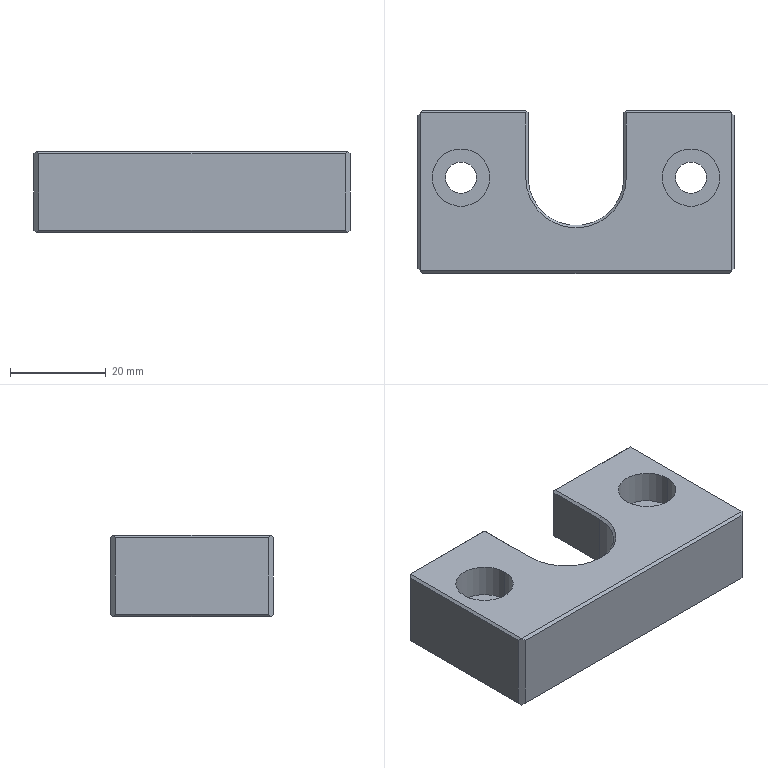Part | STEP file | 03-31SC Floating JointFixed座 | 1 solid | 51 faces | box 66 x 34 x 17 mm | volume 26495 mm3 | plane 38 | cylinder 10 | cone 3 | commonest cylinder face diameters 6.5 x4 12 x4 20 x1 31 x1
STEP:
#1=CARTESIAN_POINT('',(-30.,3.,10.));
#2=VERTEX_POINT('',#1);
#3=CARTESIAN_POINT('',(-18.,3.,10.));
#4=VERTEX_POINT('',#3);
#5=CARTESIAN_POINT('',(-24.,3.,10.));
#6=DIRECTION('',(0.,0.,1.));
#7=DIRECTION('',(1.,0.,0.));
#8=AXIS2_PLACEMENT_3D('',#5,#6,#7);
#9=CIRCLE('',#8,6.);
#10=EDGE_CURVE('',#2,#4,#9,.T.);
#11=ORIENTED_EDGE('',*,*,#10,.F.);
#12=CARTESIAN_POINT('',(-30.,3.,17.));
#13=VERTEX_POINT('',#12);
#14=CARTESIAN_POINT('',(-30.,3.,17.));
#15=DIRECTION('',(0.,0.,1.));
#16=VECTOR('',#15,1000.);
#17=LINE('',#14,#16);
#18=EDGE_CURVE('',#2,#13,#17,.T.);
#19=ORIENTED_EDGE('',*,*,#18,.T.);
#20=CARTESIAN_POINT('',(-18.,3.,17.));
#21=VERTEX_POINT('',#20);
#22=CARTESIAN_POINT('',(-24.,3.,17.));
#23=DIRECTION('',(0.,0.,1.));
#24=DIRECTION('',(1.,0.,0.));
#25=AXIS2_PLACEMENT_3D('',#22,#23,#24);
#26=CIRCLE('',#25,6.);
#27=EDGE_CURVE('',#13,#21,#26,.T.);
#28=ORIENTED_EDGE('',*,*,#27,.T.);
#29=CARTESIAN_POINT('',(-18.,3.,17.));
#30=DIRECTION('',(0.,0.,1.));
#31=VECTOR('',#30,1000.);
#32=LINE('',#29,#31);
#33=EDGE_CURVE('',#4,#21,#32,.T.);
#34=ORIENTED_EDGE('',*,*,#33,.F.);
#35=EDGE_LOOP('',(#11,#19,#28,#34));
#36=FACE_OUTER_BOUND('',#35,.T.);
#37=CARTESIAN_POINT('',(-24.,3.,17.));
#38=DIRECTION('',(0.,0.,1.));
#39=DIRECTION('',(1.,0.,0.));
#40=AXIS2_PLACEMENT_3D('',#37,#38,#39);
#41=CYLINDRICAL_SURFACE('',#40,6.);
#42=ADVANCED_FACE('',(#36),#41,.F.);
#43=CARTESIAN_POINT('',(-27.25,3.,0.));
#44=VERTEX_POINT('',#43);
#45=CARTESIAN_POINT('',(-20.75,3.,0.));
#46=VERTEX_POINT('',#45);
#47=CARTESIAN_POINT('',(-24.,3.,0.));
#48=DIRECTION('',(0.,0.,1.));
#49=DIRECTION('',(1.,0.,0.));
#50=AXIS2_PLACEMENT_3D('',#47,#48,#49);
#51=CIRCLE('',#50,3.25);
#52=EDGE_CURVE('',#44,#46,#51,.T.);
#53=ORIENTED_EDGE('',*,*,#52,.F.);
#54=CARTESIAN_POINT('',(-27.25,3.,10.));
#55=VERTEX_POINT('',#54);
#56=CARTESIAN_POINT('',(-27.25,3.,17.));
#57=DIRECTION('',(0.,0.,1.));
#58=VECTOR('',#57,1000.);
#59=LINE('',#56,#58);
#60=EDGE_CURVE('',#44,#55,#59,.T.);
#61=ORIENTED_EDGE('',*,*,#60,.T.);
#62=CARTESIAN_POINT('',(-20.75,3.,10.));
#63=VERTEX_POINT('',#62);
#64=CARTESIAN_POINT('',(-24.,3.,10.));
#65=DIRECTION('',(0.,0.,1.));
#66=DIRECTION('',(1.,0.,0.));
#67=AXIS2_PLACEMENT_3D('',#64,#65,#66);
#68=CIRCLE('',#67,3.25);
#69=EDGE_CURVE('',#55,#63,#68,.T.);
#70=ORIENTED_EDGE('',*,*,#69,.T.);
#71=CARTESIAN_POINT('',(-20.75,3.,17.));
#72=DIRECTION('',(0.,0.,1.));
#73=VECTOR('',#72,1000.);
#74=LINE('',#71,#73);
#75=EDGE_CURVE('',#46,#63,#74,.T.);
#76=ORIENTED_EDGE('',*,*,#75,.F.);
#77=EDGE_LOOP('',(#53,#61,#70,#76));
#78=FACE_OUTER_BOUND('',#77,.T.);
#79=CARTESIAN_POINT('',(-24.,3.,17.));
#80=DIRECTION('',(0.,0.,1.));
#81=DIRECTION('',(1.,0.,0.));
#82=AXIS2_PLACEMENT_3D('',#79,#80,#81);
#83=CYLINDRICAL_SURFACE('',#82,3.25);
#84=ADVANCED_FACE('',(#78),#83,.F.);
#85=CARTESIAN_POINT('',(18.,3.,10.));
#86=VERTEX_POINT('',#85);
#87=CARTESIAN_POINT('',(30.,3.,10.));
#88=VERTEX_POINT('',#87);
#89=CARTESIAN_POINT('',(24.,3.,10.));
#90=DIRECTION('',(0.,0.,1.));
#91=DIRECTION('',(1.,0.,0.));
#92=AXIS2_PLACEMENT_3D('',#89,#90,#91);
#93=CIRCLE('',#92,6.);
#94=EDGE_CURVE('',#86,#88,#93,.T.);
#95=ORIENTED_EDGE('',*,*,#94,.F.);
#96=CARTESIAN_POINT('',(18.,3.,17.));
#97=VERTEX_POINT('',#96);
#98=CARTESIAN_POINT('',(18.,3.,17.));
#99=DIRECTION('',(0.,0.,1.));
#100=VECTOR('',#99,1000.);
#101=LINE('',#98,#100);
#102=EDGE_CURVE('',#86,#97,#101,.T.);
#103=ORIENTED_EDGE('',*,*,#102,.T.);
#104=CARTESIAN_POINT('',(30.,3.,17.));
#105=VERTEX_POINT('',#104);
#106=CARTESIAN_POINT('',(24.,3.,17.));
#107=DIRECTION('',(0.,0.,1.));
#108=DIRECTION('',(1.,0.,0.));
#109=AXIS2_PLACEMENT_3D('',#106,#107,#108);
#110=CIRCLE('',#109,6.);
#111=EDGE_CURVE('',#97,#105,#110,.T.);
#112=ORIENTED_EDGE('',*,*,#111,.T.);
#113=CARTESIAN_POINT('',(30.,3.,17.));
#114=DIRECTION('',(0.,0.,1.));
#115=VECTOR('',#114,1000.);
#116=LINE('',#113,#115);
#117=EDGE_CURVE('',#88,#105,#116,.T.);
#118=ORIENTED_EDGE('',*,*,#117,.F.);
#119=EDGE_LOOP('',(#95,#103,#112,#118));
#120=FACE_OUTER_BOUND('',#119,.T.);
#121=CARTESIAN_POINT('',(24.,3.,17.));
#122=DIRECTION('',(0.,0.,1.));
#123=DIRECTION('',(1.,0.,0.));
#124=AXIS2_PLACEMENT_3D('',#121,#122,#123);
#125=CYLINDRICAL_SURFACE('',#124,6.);
#126=ADVANCED_FACE('',(#120),#125,.F.);
#127=CARTESIAN_POINT('',(20.75,3.,0.));
#128=VERTEX_POINT('',#127);
#129=CARTESIAN_POINT('',(27.25,3.,0.));
#130=VERTEX_POINT('',#129);
#131=CARTESIAN_POINT('',(24.,3.,0.));
#132=DIRECTION('',(0.,0.,1.));
#133=DIRECTION('',(1.,0.,0.));
#134=AXIS2_PLACEMENT_3D('',#131,#132,#133);
#135=CIRCLE('',#134,3.25);
#136=EDGE_CURVE('',#128,#130,#135,.T.);
#137=ORIENTED_EDGE('',*,*,#136,.F.);
#138=CARTESIAN_POINT('',(20.75,3.,10.));
#139=VERTEX_POINT('',#138);
#140=CARTESIAN_POINT('',(20.75,3.,17.));
#141=DIRECTION('',(0.,0.,1.));
#142=VECTOR('',#141,1000.);
#143=LINE('',#140,#142);
#144=EDGE_CURVE('',#128,#139,#143,.T.);
#145=ORIENTED_EDGE('',*,*,#144,.T.);
#146=CARTESIAN_POINT('',(27.25,3.,10.));
#147=VERTEX_POINT('',#146);
#148=CARTESIAN_POINT('',(24.,3.,10.));
#149=DIRECTION('',(0.,0.,1.));
#150=DIRECTION('',(1.,0.,0.));
#151=AXIS2_PLACEMENT_3D('',#148,#149,#150);
#152=CIRCLE('',#151,3.25);
#153=EDGE_CURVE('',#139,#147,#152,.T.);
#154=ORIENTED_EDGE('',*,*,#153,.T.);
#155=CARTESIAN_POINT('',(27.25,3.,17.));
#156=DIRECTION('',(0.,0.,1.));
#157=VECTOR('',#156,1000.);
#158=LINE('',#155,#157);
#159=EDGE_CURVE('',#130,#147,#158,.T.);
#160=ORIENTED_EDGE('',*,*,#159,.F.);
#161=EDGE_LOOP('',(#137,#145,#154,#160));
#162=FACE_OUTER_BOUND('',#161,.T.);
#163=CARTESIAN_POINT('',(24.,3.,17.));
#164=DIRECTION('',(0.,0.,1.));
#165=DIRECTION('',(1.,0.,0.));
#166=AXIS2_PLACEMENT_3D('',#163,#164,#165);
#167=CYLINDRICAL_SURFACE('',#166,3.25);
#168=ADVANCED_FACE('',(#162),#167,.F.);
#169=CARTESIAN_POINT('',(10.5,17.,5.));
#170=VERTEX_POINT('',#169);
#171=CARTESIAN_POINT('',(10.5,17.,16.5));
#172=VERTEX_POINT('',#171);
#173=CARTESIAN_POINT('',(10.5,17.,0.));
#174=DIRECTION('',(0.,0.,1.));
#175=VECTOR('',#174,1000.);
#176=LINE('',#173,#175);
#177=EDGE_CURVE('',#170,#172,#176,.T.);
#178=ORIENTED_EDGE('',*,*,#177,.T.);
#179=CARTESIAN_POINT('',(32.,17.,16.5));
#180=VERTEX_POINT('',#179);
#181=CARTESIAN_POINT('',(32.,17.,16.5));
#182=DIRECTION('',(1.,0.,0.));
#183=VECTOR('',#182,1000.);
#184=LINE('',#181,#183);
#185=EDGE_CURVE('',#172,#180,#184,.T.);
#186=ORIENTED_EDGE('',*,*,#185,.T.);
#187=CARTESIAN_POINT('',(32.,17.,0.5));
#188=VERTEX_POINT('',#187);
#189=CARTESIAN_POINT('',(32.,17.,17.));
#190=DIRECTION('',(0.,0.,-1.));
#191=VECTOR('',#190,1000.);
#192=LINE('',#189,#191);
#193=EDGE_CURVE('',#180,#188,#192,.T.);
#194=ORIENTED_EDGE('',*,*,#193,.T.);
#195=CARTESIAN_POINT('',(16.,17.,0.5));
#196=VERTEX_POINT('',#195);
#197=CARTESIAN_POINT('',(-32.,17.,0.5));
#198=DIRECTION('',(-1.,0.,0.));
#199=VECTOR('',#198,1000.);
#200=LINE('',#197,#199);
#201=EDGE_CURVE('',#188,#196,#200,.T.);
#202=ORIENTED_EDGE('',*,*,#201,.T.);
#203=CARTESIAN_POINT('',(16.,17.,5.));
#204=VERTEX_POINT('',#203);
#205=CARTESIAN_POINT('',(16.,17.,5.));
#206=DIRECTION('',(0.,0.,1.));
#207=VECTOR('',#206,1000.);
#208=LINE('',#205,#207);
#209=EDGE_CURVE('',#196,#204,#208,.T.);
#210=ORIENTED_EDGE('',*,*,#209,.T.);
#211=CARTESIAN_POINT('',(-15.5,17.,5.));
#212=DIRECTION('',(1.,0.,0.));
#213=VECTOR('',#212,1000.);
#214=LINE('',#211,#213);
#215=EDGE_CURVE('',#170,#204,#214,.T.);
#216=ORIENTED_EDGE('',*,*,#215,.F.);
#217=EDGE_LOOP('',(#178,#186,#194,#202,#210,#216));
#218=FACE_OUTER_BOUND('',#217,.T.);
#219=CARTESIAN_POINT('',(-32.,17.,17.));
#220=DIRECTION('',(0.,1.,0.));
#221=DIRECTION('',(-1.,0.,0.));
#222=AXIS2_PLACEMENT_3D('',#219,#220,#221);
#223=PLANE('',#222);
#224=ADVANCED_FACE('',(#218),#223,.T.);
#225=CARTESIAN_POINT('',(-32.,17.,16.5));
#226=VERTEX_POINT('',#225);
#227=CARTESIAN_POINT('',(-32.,17.,0.5));
#228=VERTEX_POINT('',#227);
#229=CARTESIAN_POINT('',(-32.,17.,17.));
#230=DIRECTION('',(0.,0.,-1.));
#231=VECTOR('',#230,1000.);
#232=LINE('',#229,#231);
#233=EDGE_CURVE('',#226,#228,#232,.T.);
#234=ORIENTED_EDGE('',*,*,#233,.T.);
#235=CARTESIAN_POINT('',(-32.5,16.5,0.));
#236=VERTEX_POINT('',#235);
#237=CARTESIAN_POINT('',(-27.167,21.833,5.333));
#238=DIRECTION('',(-0.5774,-0.5774,-0.5774));
#239=VECTOR('',#238,1000.);
#240=LINE('',#237,#239);
#241=EDGE_CURVE('',#228,#236,#240,.T.);
#242=ORIENTED_EDGE('',*,*,#241,.T.);
#243=CARTESIAN_POINT('',(-33.,16.,0.5));
#244=VERTEX_POINT('',#243);
#245=CARTESIAN_POINT('',(-38.5,10.5,6.));
#246=DIRECTION('',(-0.5774,-0.5774,0.5774));
#247=VECTOR('',#246,1000.);
#248=LINE('',#245,#247);
#249=EDGE_CURVE('',#236,#244,#248,.T.);
#250=ORIENTED_EDGE('',*,*,#249,.T.);
#251=CARTESIAN_POINT('',(-33.,16.,16.5));
#252=VERTEX_POINT('',#251);
#253=CARTESIAN_POINT('',(-33.,16.,17.));
#254=DIRECTION('',(0.,0.,-1.));
#255=VECTOR('',#254,1000.);
#256=LINE('',#253,#255);
#257=EDGE_CURVE('',#252,#244,#256,.T.);
#258=ORIENTED_EDGE('',*,*,#257,.F.);
#259=CARTESIAN_POINT('',(-32.5,16.5,17.));
#260=VERTEX_POINT('',#259);
#261=CARTESIAN_POINT('',(-32.833,16.167,16.667));
#262=DIRECTION('',(0.5774,0.5774,0.5774));
#263=VECTOR('',#262,1000.);
#264=LINE('',#261,#263);
#265=EDGE_CURVE('',#252,#260,#264,.T.);
#266=ORIENTED_EDGE('',*,*,#265,.T.);
#267=CARTESIAN_POINT('',(-32.833,16.167,17.333));
#268=DIRECTION('',(0.5774,0.5774,-0.5774));
#269=VECTOR('',#268,1000.);
#270=LINE('',#267,#269);
#271=EDGE_CURVE('',#260,#226,#270,.T.);
#272=ORIENTED_EDGE('',*,*,#271,.T.);
#273=EDGE_LOOP('',(#234,#242,#250,#258,#266,#272));
#274=FACE_OUTER_BOUND('',#273,.T.);
#275=CARTESIAN_POINT('',(-33.,16.,17.));
#276=DIRECTION('',(-0.7071,0.7071,0.));
#277=DIRECTION('',(-0.7071,-0.7071,0.));
#278=AXIS2_PLACEMENT_3D('',#275,#276,#277);
#279=PLANE('',#278);
#280=ADVANCED_FACE('',(#274),#279,.T.);
#281=ORIENTED_EDGE('',*,*,#257,.T.);
#282=CARTESIAN_POINT('',(-33.,-16.,0.5));
#283=VERTEX_POINT('',#282);
#284=CARTESIAN_POINT('',(-33.,-16.,0.5));
#285=DIRECTION('',(0.,-1.,0.));
#286=VECTOR('',#285,1000.);
#287=LINE('',#284,#286);
#288=EDGE_CURVE('',#244,#283,#287,.T.);
#289=ORIENTED_EDGE('',*,*,#288,.T.);
#290=CARTESIAN_POINT('',(-33.,-16.,16.5));
#291=VERTEX_POINT('',#290);
#292=CARTESIAN_POINT('',(-33.,-16.,17.));
#293=DIRECTION('',(0.,0.,-1.));
#294=VECTOR('',#293,1000.);
#295=LINE('',#292,#294);
#296=EDGE_CURVE('',#291,#283,#295,.T.);
#297=ORIENTED_EDGE('',*,*,#296,.F.);
#298=CARTESIAN_POINT('',(-33.,16.,16.5));
#299=DIRECTION('',(0.,1.,0.));
#300=VECTOR('',#299,1000.);
#301=LINE('',#298,#300);
#302=EDGE_CURVE('',#291,#252,#301,.T.);
#303=ORIENTED_EDGE('',*,*,#302,.T.);
#304=EDGE_LOOP('',(#281,#289,#297,#303));
#305=FACE_OUTER_BOUND('',#304,.T.);
#306=CARTESIAN_POINT('',(-33.,-16.,17.));
#307=DIRECTION('',(-1.,0.,0.));
#308=DIRECTION('',(0.,0.,1.));
#309=AXIS2_PLACEMENT_3D('',#306,#307,#308);
#310=PLANE('',#309);
#311=ADVANCED_FACE('',(#305),#310,.T.);
#312=CARTESIAN_POINT('',(-32.,-17.,16.5));
#313=VERTEX_POINT('',#312);
#314=CARTESIAN_POINT('',(-32.,-17.,0.5));
#315=VERTEX_POINT('',#314);
#316=CARTESIAN_POINT('',(-32.,-17.,17.));
#317=DIRECTION('',(0.,0.,-1.));
#318=VECTOR('',#317,1000.);
#319=LINE('',#316,#318);
#320=EDGE_CURVE('',#313,#315,#319,.T.);
#321=ORIENTED_EDGE('',*,*,#320,.F.);
#322=CARTESIAN_POINT('',(-32.5,-16.5,17.));
#323=VERTEX_POINT('',#322);
#324=CARTESIAN_POINT('',(-32.167,-16.833,16.667));
#325=DIRECTION('',(-0.5774,0.5774,0.5774));
#326=VECTOR('',#325,1000.);
#327=LINE('',#324,#326);
#328=EDGE_CURVE('',#313,#323,#327,.T.);
#329=ORIENTED_EDGE('',*,*,#328,.T.);
#330=CARTESIAN_POINT('',(-32.167,-16.833,17.333));
#331=DIRECTION('',(-0.5774,0.5774,-0.5774));
#332=VECTOR('',#331,1000.);
#333=LINE('',#330,#332);
#334=EDGE_CURVE('',#323,#291,#333,.T.);
#335=ORIENTED_EDGE('',*,*,#334,.T.);
#336=ORIENTED_EDGE('',*,*,#296,.T.);
#337=CARTESIAN_POINT('',(-32.5,-16.5,0.));
#338=VERTEX_POINT('',#337);
#339=CARTESIAN_POINT('',(-37.833,-11.167,5.333));
#340=DIRECTION('',(0.5774,-0.5774,-0.5774));
#341=VECTOR('',#340,1000.);
#342=LINE('',#339,#341);
#343=EDGE_CURVE('',#283,#338,#342,.T.);
#344=ORIENTED_EDGE('',*,*,#343,.T.);
#345=CARTESIAN_POINT('',(-26.5,-22.5,6.));
#346=DIRECTION('',(0.5774,-0.5774,0.5774));
#347=VECTOR('',#346,1000.);
#348=LINE('',#345,#347);
#349=EDGE_CURVE('',#338,#315,#348,.T.);
#350=ORIENTED_EDGE('',*,*,#349,.T.);
#351=EDGE_LOOP('',(#321,#329,#335,#336,#344,#350));
#352=FACE_OUTER_BOUND('',#351,.T.);
#353=CARTESIAN_POINT('',(-32.,-17.,17.));
#354=DIRECTION('',(-0.7071,-0.7071,0.));
#355=DIRECTION('',(0.7071,-0.7071,0.));
#356=AXIS2_PLACEMENT_3D('',#353,#354,#355);
#357=PLANE('',#356);
#358=ADVANCED_FACE('',(#352),#357,.T.);
#359=CARTESIAN_POINT('',(32.,-17.,16.5));
#360=VERTEX_POINT('',#359);
#361=CARTESIAN_POINT('',(32.,-17.,0.5));
#362=VERTEX_POINT('',#361);
#363=CARTESIAN_POINT('',(32.,-17.,17.));
#364=DIRECTION('',(0.,0.,-1.));
#365=VECTOR('',#364,1000.);
#366=LINE('',#363,#365);
#367=EDGE_CURVE('',#360,#362,#366,.T.);
#368=ORIENTED_EDGE('',*,*,#367,.F.);
#369=CARTESIAN_POINT('',(-32.,-17.,16.5));
#370=DIRECTION('',(-1.,0.,0.));
#371=VECTOR('',#370,1000.);
#372=LINE('',#369,#371);
#373=EDGE_CURVE('',#360,#313,#372,.T.);
#374=ORIENTED_EDGE('',*,*,#373,.T.);
#375=ORIENTED_EDGE('',*,*,#320,.T.);
#376=CARTESIAN_POINT('',(32.,-17.,0.5));
#377=DIRECTION('',(1.,0.,0.));
#378=VECTOR('',#377,1000.);
#379=LINE('',#376,#378);
#380=EDGE_CURVE('',#315,#362,#379,.T.);
#381=ORIENTED_EDGE('',*,*,#380,.T.);
#382=EDGE_LOOP('',(#368,#374,#375,#381));
#383=FACE_OUTER_BOUND('',#382,.T.);
#384=CARTESIAN_POINT('',(32.,-17.,17.));
#385=DIRECTION('',(0.,-1.,0.));
#386=DIRECTION('',(1.,0.,0.));
#387=AXIS2_PLACEMENT_3D('',#384,#385,#386);
#388=PLANE('',#387);
#389=ADVANCED_FACE('',(#383),#388,.T.);
#390=CARTESIAN_POINT('',(33.,-16.,16.5));
#391=VERTEX_POINT('',#390);
#392=CARTESIAN_POINT('',(32.5,-16.5,17.));
#393=VERTEX_POINT('',#392);
#394=CARTESIAN_POINT('',(32.833,-16.167,16.667));
#395=DIRECTION('',(-0.5774,-0.5774,0.5774));
#396=VECTOR('',#395,1000.);
#397=LINE('',#394,#396);
#398=EDGE_CURVE('',#391,#393,#397,.T.);
#399=ORIENTED_EDGE('',*,*,#398,.T.);
#400=CARTESIAN_POINT('',(32.833,-16.167,17.333));
#401=DIRECTION('',(-0.5774,-0.5774,-0.5774));
#402=VECTOR('',#401,1000.);
#403=LINE('',#400,#402);
#404=EDGE_CURVE('',#393,#360,#403,.T.);
#405=ORIENTED_EDGE('',*,*,#404,.T.);
#406=ORIENTED_EDGE('',*,*,#367,.T.);
#407=CARTESIAN_POINT('',(32.5,-16.5,0.));
#408=VERTEX_POINT('',#407);
#409=CARTESIAN_POINT('',(27.167,-21.833,5.333));
#410=DIRECTION('',(0.5774,0.5774,-0.5774));
#411=VECTOR('',#410,1000.);
#412=LINE('',#409,#411);
#413=EDGE_CURVE('',#362,#408,#412,.T.);
#414=ORIENTED_EDGE('',*,*,#413,.T.);
#415=CARTESIAN_POINT('',(33.,-16.,0.5));
#416=VERTEX_POINT('',#415);
#417=CARTESIAN_POINT('',(38.5,-10.5,6.));
#418=DIRECTION('',(0.5774,0.5774,0.5774));
#419=VECTOR('',#418,1000.);
#420=LINE('',#417,#419);
#421=EDGE_CURVE('',#408,#416,#420,.T.);
#422=ORIENTED_EDGE('',*,*,#421,.T.);
#423=CARTESIAN_POINT('',(33.,-16.,17.));
#424=DIRECTION('',(0.,0.,-1.));
#425=VECTOR('',#424,1000.);
#426=LINE('',#423,#425);
#427=EDGE_CURVE('',#391,#416,#426,.T.);
#428=ORIENTED_EDGE('',*,*,#427,.F.);
#429=EDGE_LOOP('',(#399,#405,#406,#414,#422,#428));
#430=FACE_OUTER_BOUND('',#429,.T.);
#431=CARTESIAN_POINT('',(33.,-16.,17.));
#432=DIRECTION('',(0.7071,-0.7071,0.));
#433=DIRECTION('',(0.7071,0.7071,0.));
#434=AXIS2_PLACEMENT_3D('',#431,#432,#433);
#435=PLANE('',#434);
#436=ADVANCED_FACE('',(#430),#435,.T.);
#437=CARTESIAN_POINT('',(33.,16.,16.5));
#438=VERTEX_POINT('',#437);
#439=CARTESIAN_POINT('',(33.,16.,0.5));
#440=VERTEX_POINT('',#439);
#441=CARTESIAN_POINT('',(33.,16.,17.));
#442=DIRECTION('',(0.,0.,-1.));
#443=VECTOR('',#442,1000.);
#444=LINE('',#441,#443);
#445=EDGE_CURVE('',#438,#440,#444,.T.);
#446=ORIENTED_EDGE('',*,*,#445,.F.);
#447=CARTESIAN_POINT('',(33.,-16.,16.5));
#448=DIRECTION('',(0.,-1.,0.));
#449=VECTOR('',#448,1000.);
#450=LINE('',#447,#449);
#451=EDGE_CURVE('',#438,#391,#450,.T.);
#452=ORIENTED_EDGE('',*,*,#451,.T.);
#453=ORIENTED_EDGE('',*,*,#427,.T.);
#454=CARTESIAN_POINT('',(33.,16.,0.5));
#455=DIRECTION('',(0.,1.,0.));
#456=VECTOR('',#455,1000.);
#457=LINE('',#454,#456);
#458=EDGE_CURVE('',#416,#440,#457,.T.);
#459=ORIENTED_EDGE('',*,*,#458,.T.);
#460=EDGE_LOOP('',(#446,#452,#453,#459));
#461=FACE_OUTER_BOUND('',#460,.T.);
#462=CARTESIAN_POINT('',(33.,16.,17.));
#463=DIRECTION('',(1.,0.,0.));
#464=DIRECTION('',(0.,0.,-1.));
#465=AXIS2_PLACEMENT_3D('',#462,#463,#464);
#466=PLANE('',#465);
#467=ADVANCED_FACE('',(#461),#466,.T.);
#468=ORIENTED_EDGE('',*,*,#193,.F.);
#469=CARTESIAN_POINT('',(32.5,16.5,17.));
#470=VERTEX_POINT('',#469);
#471=CARTESIAN_POINT('',(32.167,16.833,16.667));
#472=DIRECTION('',(0.5774,-0.5774,0.5774));
#473=VECTOR('',#472,1000.);
#474=LINE('',#471,#473);
#475=EDGE_CURVE('',#180,#470,#474,.T.);
#476=ORIENTED_EDGE('',*,*,#475,.T.);
#477=CARTESIAN_POINT('',(32.167,16.833,17.333));
#478=DIRECTION('',(0.5774,-0.5774,-0.5774));
#479=VECTOR('',#478,1000.);
#480=LINE('',#477,#479);
#481=EDGE_CURVE('',#470,#438,#480,.T.);
#482=ORIENTED_EDGE('',*,*,#481,.T.);
#483=ORIENTED_EDGE('',*,*,#445,.T.);
#484=CARTESIAN_POINT('',(32.5,16.5,0.));
#485=VERTEX_POINT('',#484);
#486=CARTESIAN_POINT('',(37.833,11.167,5.333));
#487=DIRECTION('',(-0.5774,0.5774,-0.5774));
#488=VECTOR('',#487,1000.);
#489=LINE('',#486,#488);
#490=EDGE_CURVE('',#440,#485,#489,.T.);
#491=ORIENTED_EDGE('',*,*,#490,.T.);
#492=CARTESIAN_POINT('',(26.5,22.5,6.));
#493=DIRECTION('',(-0.5774,0.5774,0.5774));
#494=VECTOR('',#493,1000.);
#495=LINE('',#492,#494);
#496=EDGE_CURVE('',#485,#188,#495,.T.);
#497=ORIENTED_EDGE('',*,*,#496,.T.);
#498=EDGE_LOOP('',(#468,#476,#482,#483,#491,#497));
#499=FACE_OUTER_BOUND('',#498,.T.);
#500=CARTESIAN_POINT('',(32.,17.,17.));
#501=DIRECTION('',(0.7071,0.7071,0.));
#502=DIRECTION('',(-0.7071,0.7071,0.));
#503=AXIS2_PLACEMENT_3D('',#500,#501,#502);
#504=PLANE('',#503);
#505=ADVANCED_FACE('',(#499),#504,.T.);
#506=ORIENTED_EDGE('',*,*,#233,.F.);
#507=CARTESIAN_POINT('',(-10.5,17.,16.5));
#508=VERTEX_POINT('',#507);
#509=CARTESIAN_POINT('',(-10.5,17.,16.5));
#510=DIRECTION('',(1.,0.,0.));
#511=VECTOR('',#510,1000.);
#512=LINE('',#509,#511);
#513=EDGE_CURVE('',#226,#508,#512,.T.);
#514=ORIENTED_EDGE('',*,*,#513,.T.);
#515=CARTESIAN_POINT('',(-10.5,17.,5.));
#516=VERTEX_POINT('',#515);
#517=CARTESIAN_POINT('',(-10.5,17.,0.));
#518=DIRECTION('',(0.,0.,1.));
#519=VECTOR('',#518,1000.);
#520=LINE('',#517,#519);
#521=EDGE_CURVE('',#516,#508,#520,.T.);
#522=ORIENTED_EDGE('',*,*,#521,.F.);
#523=CARTESIAN_POINT('',(-16.,17.,5.));
#524=VERTEX_POINT('',#523);
#525=CARTESIAN_POINT('',(-15.5,17.,5.));
#526=DIRECTION('',(1.,0.,0.));
#527=VECTOR('',#526,1000.);
#528=LINE('',#525,#527);
#529=EDGE_CURVE('',#524,#516,#528,.T.);
#530=ORIENTED_EDGE('',*,*,#529,.F.);
#531=CARTESIAN_POINT('',(-16.,17.,0.5));
#532=VERTEX_POINT('',#531);
#533=CARTESIAN_POINT('',(-16.,17.,0.));
#534=DIRECTION('',(0.,0.,-1.));
#535=VECTOR('',#534,1000.);
#536=LINE('',#533,#535);
#537=EDGE_CURVE('',#524,#532,#536,.T.);
#538=ORIENTED_EDGE('',*,*,#537,.T.);
#539=CARTESIAN_POINT('',(-32.,17.,0.5));
#540=DIRECTION('',(-1.,0.,0.));
#541=VECTOR('',#540,1000.);
#542=LINE('',#539,#541);
#543=EDGE_CURVE('',#532,#228,#542,.T.);
#544=ORIENTED_EDGE('',*,*,#543,.T.);
#545=EDGE_LOOP('',(#506,#514,#522,#530,#538,#544));
#546=FACE_OUTER_BOUND('',#545,.T.);
#547=CARTESIAN_POINT('',(-32.,17.,17.));
#548=DIRECTION('',(0.,1.,0.));
#549=DIRECTION('',(-1.,0.,0.));
#550=AXIS2_PLACEMENT_3D('',#547,#548,#549);
#551=PLANE('',#550);
#552=ADVANCED_FACE('',(#546),#551,.T.);
#553=CARTESIAN_POINT('',(10.5,16.5,17.));
#554=VERTEX_POINT('',#553);
#555=CARTESIAN_POINT('',(10.5,16.5,17.));
#556=DIRECTION('',(-1.,0.,0.));
#557=VECTOR('',#556,1000.);
#558=LINE('',#555,#557);
#559=EDGE_CURVE('',#470,#554,#558,.T.);
#560=ORIENTED_EDGE('',*,*,#559,.T.);
#561=CARTESIAN_POINT('',(10.5,3.,17.));
#562=VERTEX_POINT('',#561);
#563=CARTESIAN_POINT('',(10.5,49.,17.));
#564=DIRECTION('',(0.,-1.,0.));
#565=VECTOR('',#564,1000.);
#566=LINE('',#563,#565);
#567=EDGE_CURVE('',#554,#562,#566,.T.);
#568=ORIENTED_EDGE('',*,*,#567,.T.);
#569=CARTESIAN_POINT('',(-10.5,3.,17.));
#570=VERTEX_POINT('',#569);
#571=CARTESIAN_POINT('',(0.,3.,17.));
#572=DIRECTION('',(0.,0.,-1.));
#573=DIRECTION('',(-1.,0.,0.));
#574=AXIS2_PLACEMENT_3D('',#571,#572,#573);
#575=CIRCLE('',#574,10.5);
#576=EDGE_CURVE('',#562,#570,#575,.T.);
#577=ORIENTED_EDGE('',*,*,#576,.T.);
#578=CARTESIAN_POINT('',(-10.5,16.5,17.));
#579=VERTEX_POINT('',#578);
#580=CARTESIAN_POINT('',(-10.5,49.,17.));
#581=DIRECTION('',(0.,1.,0.));
#582=VECTOR('',#581,1000.);
#583=LINE('',#580,#582);
#584=EDGE_CURVE('',#570,#579,#583,.T.);
#585=ORIENTED_EDGE('',*,*,#584,.T.);
#586=CARTESIAN_POINT('',(-32.,16.5,17.));
#587=DIRECTION('',(-1.,0.,0.));
#588=VECTOR('',#587,1000.);
#589=LINE('',#586,#588);
#590=EDGE_CURVE('',#579,#260,#589,.T.);
#591=ORIENTED_EDGE('',*,*,#590,.T.);
#592=CARTESIAN_POINT('',(-32.5,-16.,17.));
#593=DIRECTION('',(0.,-1.,0.));
#594=VECTOR('',#593,1000.);
#595=LINE('',#592,#594);
#596=EDGE_CURVE('',#260,#323,#595,.T.);
#597=ORIENTED_EDGE('',*,*,#596,.T.);
#598=CARTESIAN_POINT('',(32.,-16.5,17.));
#599=DIRECTION('',(1.,0.,0.));
#600=VECTOR('',#599,1000.);
#601=LINE('',#598,#600);
#602=EDGE_CURVE('',#323,#393,#601,.T.);
#603=ORIENTED_EDGE('',*,*,#602,.T.);
#604=CARTESIAN_POINT('',(32.5,16.,17.));
#605=DIRECTION('',(0.,1.,0.));
#606=VECTOR('',#605,1000.);
#607=LINE('',#604,#606);
#608=EDGE_CURVE('',#393,#470,#607,.T.);
#609=ORIENTED_EDGE('',*,*,#608,.T.);
#610=EDGE_LOOP('',(#560,#568,#577,#585,#591,#597,#603,#609));
#611=FACE_OUTER_BOUND('',#610,.T.);
#612=CARTESIAN_POINT('',(-24.,3.,17.));
#613=DIRECTION('',(0.,0.,1.));
#614=DIRECTION('',(1.,0.,0.));
#615=AXIS2_PLACEMENT_3D('',#612,#613,#614);
#616=CIRCLE('',#615,6.);
#617=EDGE_CURVE('',#21,#13,#616,.T.);
#618=ORIENTED_EDGE('',*,*,#617,.F.);
#619=ORIENTED_EDGE('',*,*,#27,.F.);
#620=EDGE_LOOP('',(#618,#619));
#621=FACE_BOUND('',#620,.T.);
#622=CARTESIAN_POINT('',(24.,3.,17.));
#623=DIRECTION('',(0.,0.,1.));
#624=DIRECTION('',(1.,0.,0.));
#625=AXIS2_PLACEMENT_3D('',#622,#623,#624);
#626=CIRCLE('',#625,6.);
#627=EDGE_CURVE('',#105,#97,#626,.T.);
#628=ORIENTED_EDGE('',*,*,#627,.F.);
#629=ORIENTED_EDGE('',*,*,#111,.F.);
#630=EDGE_LOOP('',(#628,#629));
#631=FACE_BOUND('',#630,.T.);
#632=CARTESIAN_POINT('',(0.,49.,17.));
#633=DIRECTION('',(0.,0.,-1.));
#634=DIRECTION('',(-1.,0.,0.));
#635=AXIS2_PLACEMENT_3D('',#632,#633,#634);
#636=PLANE('',#635);
#637=ADVANCED_FACE('',(#611,#621,#631),#636,.F.);
#638=CARTESIAN_POINT('',(-16.,16.5,0.));
#639=VERTEX_POINT('',#638);
#640=CARTESIAN_POINT('',(0.,16.5,0.));
#641=DIRECTION('',(1.,0.,0.));
#642=VECTOR('',#641,1000.);
#643=LINE('',#640,#642);
#644=EDGE_CURVE('',#236,#639,#643,.T.);
#645=ORIENTED_EDGE('',*,*,#644,.T.);
#646=CARTESIAN_POINT('',(-16.,3.,0.));
#647=VERTEX_POINT('',#646);
#648=CARTESIAN_POINT('',(-16.,3.,0.));
#649=DIRECTION('',(0.,-1.,0.));
#650=VECTOR('',#649,1000.);
#651=LINE('',#648,#650);
#652=EDGE_CURVE('',#639,#647,#651,.T.);
#653=ORIENTED_EDGE('',*,*,#652,.T.);
#654=CARTESIAN_POINT('',(16.,3.,0.));
#655=VERTEX_POINT('',#654);
#656=CARTESIAN_POINT('',(0.,3.,0.));
#657=DIRECTION('',(0.,0.,1.));
#658=DIRECTION('',(-1.,0.,0.));
#659=AXIS2_PLACEMENT_3D('',#656,#657,#658);
#660=CIRCLE('',#659,16.);
#661=EDGE_CURVE('',#647,#655,#660,.T.);
#662=ORIENTED_EDGE('',*,*,#661,.T.);
#663=CARTESIAN_POINT('',(16.,16.5,0.));
#664=VERTEX_POINT('',#663);
#665=CARTESIAN_POINT('',(16.,16.5,0.));
#666=DIRECTION('',(0.,1.,0.));
#667=VECTOR('',#666,1000.);
#668=LINE('',#665,#667);
#669=EDGE_CURVE('',#655,#664,#668,.T.);
#670=ORIENTED_EDGE('',*,*,#669,.T.);
#671=CARTESIAN_POINT('',(0.,16.5,0.));
#672=DIRECTION('',(1.,0.,0.));
#673=VECTOR('',#672,1000.);
#674=LINE('',#671,#673);
#675=EDGE_CURVE('',#664,#485,#674,.T.);
#676=ORIENTED_EDGE('',*,*,#675,.T.);
#677=CARTESIAN_POINT('',(32.5,49.,0.));
#678=DIRECTION('',(0.,-1.,0.));
#679=VECTOR('',#678,1000.);
#680=LINE('',#677,#679);
#681=EDGE_CURVE('',#485,#408,#680,.T.);
#682=ORIENTED_EDGE('',*,*,#681,.T.);
#683=CARTESIAN_POINT('',(0.,-16.5,0.));
#684=DIRECTION('',(-1.,0.,0.));
#685=VECTOR('',#684,1000.);
#686=LINE('',#683,#685);
#687=EDGE_CURVE('',#408,#338,#686,.T.);
#688=ORIENTED_EDGE('',*,*,#687,.T.);
#689=CARTESIAN_POINT('',(-32.5,49.,0.));
#690=DIRECTION('',(0.,1.,0.));
#691=VECTOR('',#690,1000.);
#692=LINE('',#689,#691);
#693=EDGE_CURVE('',#338,#236,#692,.T.);
#694=ORIENTED_EDGE('',*,*,#693,.T.);
#695=EDGE_LOOP('',(#645,#653,#662,#670,#676,#682,#688,#694));
#696=FACE_OUTER_BOUND('',#695,.T.);
#697=CARTESIAN_POINT('',(-24.,3.,0.));
#698=DIRECTION('',(0.,0.,1.));
#699=DIRECTION('',(1.,0.,0.));
#700=AXIS2_PLACEMENT_3D('',#697,#698,#699);
#701=CIRCLE('',#700,3.25);
#702=EDGE_CURVE('',#46,#44,#701,.T.);
#703=ORIENTED_EDGE('',*,*,#702,.T.);
#704=ORIENTED_EDGE('',*,*,#52,.T.);
#705=EDGE_LOOP('',(#703,#704));
#706=FACE_BOUND('',#705,.T.);
#707=CARTESIAN_POINT('',(24.,3.,0.));
#708=DIRECTION('',(0.,0.,1.));
#709=DIRECTION('',(1.,0.,0.));
#710=AXIS2_PLACEMENT_3D('',#707,#708,#709);
#711=CIRCLE('',#710,3.25);
#712=EDGE_CURVE('',#130,#128,#711,.T.);
#713=ORIENTED_EDGE('',*,*,#712,.T.);
#714=ORIENTED_EDGE('',*,*,#136,.T.);
#715=EDGE_LOOP('',(#713,#714));
#716=FACE_BOUND('',#715,.T.);
#717=CARTESIAN_POINT('',(0.,49.,0.));
#718=DIRECTION('',(0.,0.,-1.));
#719=DIRECTION('',(-1.,0.,0.));
#720=AXIS2_PLACEMENT_3D('',#717,#718,#719);
#721=PLANE('',#720);
#722=ADVANCED_FACE('',(#696,#706,#716),#721,.T.);
#723=CARTESIAN_POINT('',(-15.5,3.,5.));
#724=VERTEX_POINT('',#723);
#725=CARTESIAN_POINT('',(-15.5,3.,0.5));
#726=VERTEX_POINT('',#725);
#727=CARTESIAN_POINT('',(-15.5,3.,5.));
#728=DIRECTION('',(0.,0.,-1.));
#729=VECTOR('',#728,1000.);
#730=LINE('',#727,#729);
#731=EDGE_CURVE('',#724,#726,#730,.T.);
#732=ORIENTED_EDGE('',*,*,#731,.T.);
#733=CARTESIAN_POINT('',(-15.5,16.5,0.5));
#734=VERTEX_POINT('',#733);
#735=CARTESIAN_POINT('',(-15.5,16.5,0.5));
#736=DIRECTION('',(0.,1.,0.));
#737=VECTOR('',#736,1000.);
#738=LINE('',#735,#737);
#739=EDGE_CURVE('',#726,#734,#738,.T.);
#740=ORIENTED_EDGE('',*,*,#739,.T.);
#741=CARTESIAN_POINT('',(-15.5,16.5,5.));
#742=VERTEX_POINT('',#741);
#743=CARTESIAN_POINT('',(-15.5,16.5,5.));
#744=DIRECTION('',(0.,0.,1.));
#745=VECTOR('',#744,1000.);
#746=LINE('',#743,#745);
#747=EDGE_CURVE('',#734,#742,#746,.T.);
#748=ORIENTED_EDGE('',*,*,#747,.T.);
#749=CARTESIAN_POINT('',(-15.5,3.,5.));
#750=DIRECTION('',(0.,1.,0.));
#751=VECTOR('',#750,1000.);
#752=LINE('',#749,#751);
#753=EDGE_CURVE('',#724,#742,#752,.T.);
#754=ORIENTED_EDGE('',*,*,#753,.F.);
#755=EDGE_LOOP('',(#732,#740,#748,#754));
#756=FACE_OUTER_BOUND('',#755,.T.);
#757=CARTESIAN_POINT('',(-15.5,3.,5.));
#758=DIRECTION('',(-1.,0.,0.));
#759=DIRECTION('',(0.,0.,1.));
#760=AXIS2_PLACEMENT_3D('',#757,#758,#759);
#761=PLANE('',#760);
#762=ADVANCED_FACE('',(#756),#761,.F.);
#763=CARTESIAN_POINT('',(15.5,3.,5.));
#764=VERTEX_POINT('',#763);
#765=CARTESIAN_POINT('',(15.5,3.,0.5));
#766=VERTEX_POINT('',#765);
#767=CARTESIAN_POINT('',(15.5,3.,5.));
#768=DIRECTION('',(0.,0.,-1.));
#769=VECTOR('',#768,1000.);
#770=LINE('',#767,#769);
#771=EDGE_CURVE('',#764,#766,#770,.T.);
#772=ORIENTED_EDGE('',*,*,#771,.T.);
#773=CARTESIAN_POINT('',(0.,3.,0.5));
#774=DIRECTION('',(0.,0.,-1.));
#775=DIRECTION('',(-1.,0.,0.));
#776=AXIS2_PLACEMENT_3D('',#773,#774,#775);
#777=CIRCLE('',#776,15.5);
#778=EDGE_CURVE('',#766,#726,#777,.T.);
#779=ORIENTED_EDGE('',*,*,#778,.T.);
#780=ORIENTED_EDGE('',*,*,#731,.F.);
#781=CARTESIAN_POINT('',(0.,3.,5.));
#782=DIRECTION('',(0.,0.,-1.));
#783=DIRECTION('',(-1.,0.,0.));
#784=AXIS2_PLACEMENT_3D('',#781,#782,#783);
#785=CIRCLE('',#784,15.5);
#786=EDGE_CURVE('',#764,#724,#785,.T.);
#787=ORIENTED_EDGE('',*,*,#786,.F.);
#788=EDGE_LOOP('',(#772,#779,#780,#787));
#789=FACE_OUTER_BOUND('',#788,.T.);
#790=CARTESIAN_POINT('',(0.,3.,5.));
#791=DIRECTION('',(0.,0.,-1.));
#792=DIRECTION('',(-1.,0.,0.));
#793=AXIS2_PLACEMENT_3D('',#790,#791,#792);
#794=CYLINDRICAL_SURFACE('',#793,15.5);
#795=ADVANCED_FACE('',(#789),#794,.F.);
#796=CARTESIAN_POINT('',(15.5,16.5,5.));
#797=VERTEX_POINT('',#796);
#798=CARTESIAN_POINT('',(15.5,16.5,0.5));
#799=VERTEX_POINT('',#798);
#800=CARTESIAN_POINT('',(15.5,16.5,0.));
#801=DIRECTION('',(0.,0.,-1.));
#802=VECTOR('',#801,1000.);
#803=LINE('',#800,#802);
#804=EDGE_CURVE('',#797,#799,#803,.T.);
#805=ORIENTED_EDGE('',*,*,#804,.T.);
#806=CARTESIAN_POINT('',(15.5,3.,0.5));
#807=DIRECTION('',(0.,-1.,0.));
#808=VECTOR('',#807,1000.);
#809=LINE('',#806,#808);
#810=EDGE_CURVE('',#799,#766,#809,.T.);
#811=ORIENTED_EDGE('',*,*,#810,.T.);
#812=ORIENTED_EDGE('',*,*,#771,.F.);
#813=CARTESIAN_POINT('',(15.5,17.,5.));
#814=DIRECTION('',(0.,-1.,0.));
#815=VECTOR('',#814,1000.);
#816=LINE('',#813,#815);
#817=EDGE_CURVE('',#797,#764,#816,.T.);
#818=ORIENTED_EDGE('',*,*,#817,.F.);
#819=EDGE_LOOP('',(#805,#811,#812,#818));
#820=FACE_OUTER_BOUND('',#819,.T.);
#821=CARTESIAN_POINT('',(15.5,17.,5.));
#822=DIRECTION('',(1.,0.,0.));
#823=DIRECTION('',(0.,0.,-1.));
#824=AXIS2_PLACEMENT_3D('',#821,#822,#823);
#825=PLANE('',#824);
#826=ADVANCED_FACE('',(#820),#825,.F.);
#827=CARTESIAN_POINT('',(-10.5,3.,5.));
#828=VERTEX_POINT('',#827);
#829=CARTESIAN_POINT('',(10.5,3.,5.));
#830=VERTEX_POINT('',#829);
#831=CARTESIAN_POINT('',(0.,3.,5.));
#832=DIRECTION('',(0.,0.,1.));
#833=DIRECTION('',(-1.,0.,0.));
#834=AXIS2_PLACEMENT_3D('',#831,#832,#833);
#835=CIRCLE('',#834,10.5);
#836=EDGE_CURVE('',#828,#830,#835,.T.);
#837=ORIENTED_EDGE('',*,*,#836,.T.);
#838=CARTESIAN_POINT('',(10.5,16.5,5.));
#839=DIRECTION('',(0.,1.,0.));
#840=VECTOR('',#839,1000.);
#841=LINE('',#838,#840);
#842=EDGE_CURVE('',#830,#170,#841,.T.);
#843=ORIENTED_EDGE('',*,*,#842,.T.);
#844=ORIENTED_EDGE('',*,*,#215,.T.);
#845=CARTESIAN_POINT('',(15.5,16.5,5.));
#846=DIRECTION('',(-0.7071,-0.7071,0.));
#847=VECTOR('',#846,1000.);
#848=LINE('',#845,#847);
#849=EDGE_CURVE('',#204,#797,#848,.T.);
#850=ORIENTED_EDGE('',*,*,#849,.T.);
#851=ORIENTED_EDGE('',*,*,#817,.T.);
#852=ORIENTED_EDGE('',*,*,#786,.T.);
#853=ORIENTED_EDGE('',*,*,#753,.T.);
#854=CARTESIAN_POINT('',(-16.,17.,5.));
#855=DIRECTION('',(-0.7071,0.7071,0.));
#856=VECTOR('',#855,1000.);
#857=LINE('',#854,#856);
#858=EDGE_CURVE('',#742,#524,#857,.T.);
#859=ORIENTED_EDGE('',*,*,#858,.T.);
#860=ORIENTED_EDGE('',*,*,#529,.T.);
#861=CARTESIAN_POINT('',(-10.5,3.,5.));
#862=DIRECTION('',(0.,-1.,0.));
#863=VECTOR('',#862,1000.);
#864=LINE('',#861,#863);
#865=EDGE_CURVE('',#516,#828,#864,.T.);
#866=ORIENTED_EDGE('',*,*,#865,.T.);
#867=EDGE_LOOP('',(#837,#843,#844,#850,#851,#852,#853,#859,#860,#866));
#868=FACE_OUTER_BOUND('',#867,.T.);
#869=CARTESIAN_POINT('',(0.,3.,5.));
#870=DIRECTION('',(0.,0.,-1.));
#871=DIRECTION('',(-1.,0.,0.));
#872=AXIS2_PLACEMENT_3D('',#869,#870,#871);
#873=PLANE('',#872);
#874=ADVANCED_FACE('',(#868),#873,.T.);
#875=ORIENTED_EDGE('',*,*,#177,.F.);
#876=CARTESIAN_POINT('',(10.,16.5,5.5));
#877=VERTEX_POINT('',#876);
#878=CARTESIAN_POINT('',(5.5,12.,10.));
#879=DIRECTION('',(-0.5774,-0.5774,0.5774));
#880=VECTOR('',#879,1000.);
#881=LINE('',#878,#880);
#882=EDGE_CURVE('',#170,#877,#881,.T.);
#883=ORIENTED_EDGE('',*,*,#882,.T.);
#884=CARTESIAN_POINT('',(10.,16.5,16.5));
#885=VERTEX_POINT('',#884);
#886=CARTESIAN_POINT('',(10.,16.5,0.));
#887=DIRECTION('',(0.,0.,1.));
#888=VECTOR('',#887,1000.);
#889=LINE('',#886,#888);
#890=EDGE_CURVE('',#877,#885,#889,.T.);
#891=ORIENTED_EDGE('',*,*,#890,.T.);
#892=CARTESIAN_POINT('',(10.25,16.75,16.75));
#893=VERTEX_POINT('',#892);
#894=CARTESIAN_POINT('',(5.5,12.,12.));
#895=DIRECTION('',(0.5774,0.5774,0.5774));
#896=VECTOR('',#895,1000.);
#897=LINE('',#894,#896);
#898=EDGE_CURVE('',#885,#893,#897,.T.);
#899=ORIENTED_EDGE('',*,*,#898,.T.);
#900=CARTESIAN_POINT('',(-3.667,2.833,30.667));
#901=DIRECTION('',(0.5774,0.5774,-0.5774));
#902=VECTOR('',#901,1000.);
#903=LINE('',#900,#902);
#904=EDGE_CURVE('',#893,#172,#903,.T.);
#905=ORIENTED_EDGE('',*,*,#904,.T.);
#906=EDGE_LOOP('',(#875,#883,#891,#899,#905));
#907=FACE_OUTER_BOUND('',#906,.T.);
#908=CARTESIAN_POINT('',(10.,16.5,0.));
#909=DIRECTION('',(0.7071,-0.7071,0.));
#910=DIRECTION('',(0.7071,0.7071,0.));
#911=AXIS2_PLACEMENT_3D('',#908,#909,#910);
#912=PLANE('',#911);
#913=ADVANCED_FACE('',(#907),#912,.F.);
#914=ORIENTED_EDGE('',*,*,#890,.F.);
#915=CARTESIAN_POINT('',(10.,3.,5.5));
#916=VERTEX_POINT('',#915);
#917=CARTESIAN_POINT('',(10.,3.,5.5));
#918=DIRECTION('',(0.,-1.,0.));
#919=VECTOR('',#918,1000.);
#920=LINE('',#917,#919);
#921=EDGE_CURVE('',#877,#916,#920,.T.);
#922=ORIENTED_EDGE('',*,*,#921,.T.);
#923=CARTESIAN_POINT('',(10.,3.,16.5));
#924=VERTEX_POINT('',#923);
#925=CARTESIAN_POINT('',(10.,3.,0.));
#926=DIRECTION('',(0.,0.,1.));
#927=VECTOR('',#926,1000.);
#928=LINE('',#925,#927);
#929=EDGE_CURVE('',#916,#924,#928,.T.);
#930=ORIENTED_EDGE('',*,*,#929,.T.);
#931=CARTESIAN_POINT('',(10.,3.,16.5));
#932=DIRECTION('',(0.,1.,0.));
#933=VECTOR('',#932,1000.);
#934=LINE('',#931,#933);
#935=EDGE_CURVE('',#924,#885,#934,.T.);
#936=ORIENTED_EDGE('',*,*,#935,.T.);
#937=EDGE_LOOP('',(#914,#922,#930,#936));
#938=FACE_OUTER_BOUND('',#937,.T.);
#939=CARTESIAN_POINT('',(10.,3.,0.));
#940=DIRECTION('',(1.,0.,0.));
#941=DIRECTION('',(0.,1.,0.));
#942=AXIS2_PLACEMENT_3D('',#939,#940,#941);
#943=PLANE('',#942);
#944=ADVANCED_FACE('',(#938),#943,.F.);
#945=ORIENTED_EDGE('',*,*,#929,.F.);
#946=CARTESIAN_POINT('',(-10.,3.,5.5));
#947=VERTEX_POINT('',#946);
#948=CARTESIAN_POINT('',(0.,3.,5.5));
#949=DIRECTION('',(0.,0.,-1.));
#950=DIRECTION('',(-1.,0.,0.));
#951=AXIS2_PLACEMENT_3D('',#948,#949,#950);
#952=CIRCLE('',#951,10.);
#953=EDGE_CURVE('',#916,#947,#952,.T.);
#954=ORIENTED_EDGE('',*,*,#953,.T.);
#955=CARTESIAN_POINT('',(-10.,3.,16.5));
#956=VERTEX_POINT('',#955);
#957=CARTESIAN_POINT('',(-10.,3.,0.));
#958=DIRECTION('',(0.,0.,1.));
#959=VECTOR('',#958,1000.);
#960=LINE('',#957,#959);
#961=EDGE_CURVE('',#947,#956,#960,.T.);
#962=ORIENTED_EDGE('',*,*,#961,.T.);
#963=CARTESIAN_POINT('',(0.,3.,16.5));
#964=DIRECTION('',(0.,0.,1.));
#965=DIRECTION('',(-1.,0.,0.));
#966=AXIS2_PLACEMENT_3D('',#963,#964,#965);
#967=CIRCLE('',#966,10.);
#968=EDGE_CURVE('',#956,#924,#967,.T.);
#969=ORIENTED_EDGE('',*,*,#968,.T.);
#970=EDGE_LOOP('',(#945,#954,#962,#969));
#971=FACE_OUTER_BOUND('',#970,.T.);
#972=CARTESIAN_POINT('',(0.,3.,0.));
#973=DIRECTION('',(0.,0.,1.));
#974=DIRECTION('',(1.,0.,0.));
#975=AXIS2_PLACEMENT_3D('',#972,#973,#974);
#976=CYLINDRICAL_SURFACE('',#975,10.);
#977=ADVANCED_FACE('',(#971),#976,.F.);
#978=ORIENTED_EDGE('',*,*,#961,.F.);
#979=CARTESIAN_POINT('',(-10.,16.5,5.5));
#980=VERTEX_POINT('',#979);
#981=CARTESIAN_POINT('',(-10.,16.5,5.5));
#982=DIRECTION('',(0.,1.,0.));
#983=VECTOR('',#982,1000.);
#984=LINE('',#981,#983);
#985=EDGE_CURVE('',#947,#980,#984,.T.);
#986=ORIENTED_EDGE('',*,*,#985,.T.);
#987=CARTESIAN_POINT('',(-10.,16.5,16.5));
#988=VERTEX_POINT('',#987);
#989=CARTESIAN_POINT('',(-10.,16.5,0.));
#990=DIRECTION('',(0.,0.,1.));
#991=VECTOR('',#990,1000.);
#992=LINE('',#989,#991);
#993=EDGE_CURVE('',#980,#988,#992,.T.);
#994=ORIENTED_EDGE('',*,*,#993,.T.);
#995=CARTESIAN_POINT('',(-10.,16.5,16.5));
#996=DIRECTION('',(0.,-1.,0.));
#997=VECTOR('',#996,1000.);
#998=LINE('',#995,#997);
#999=EDGE_CURVE('',#988,#956,#998,.T.);
#1000=ORIENTED_EDGE('',*,*,#999,.T.);
#1001=EDGE_LOOP('',(#978,#986,#994,#1000));
#1002=FACE_OUTER_BOUND('',#1001,.T.);
#1003=CARTESIAN_POINT('',(-10.,16.5,0.));
#1004=DIRECTION('',(-1.,0.,0.));
#1005=DIRECTION('',(0.,-1.,0.));
#1006=AXIS2_PLACEMENT_3D('',#1003,#1004,#1005);
#1007=PLANE('',#1006);
#1008=ADVANCED_FACE('',(#1002),#1007,.F.);
#1009=ORIENTED_EDGE('',*,*,#993,.F.);
#1010=CARTESIAN_POINT('',(-10.,16.5,5.5));
#1011=DIRECTION('',(-0.5774,0.5774,-0.5774));
#1012=VECTOR('',#1011,1000.);
#1013=LINE('',#1010,#1012);
#1014=EDGE_CURVE('',#980,#516,#1013,.T.);
#1015=ORIENTED_EDGE('',*,*,#1014,.T.);
#1016=ORIENTED_EDGE('',*,*,#521,.T.);
#1017=CARTESIAN_POINT('',(-10.25,16.75,16.75));
#1018=VERTEX_POINT('',#1017);
#1019=CARTESIAN_POINT('',(-17.667,24.167,9.333));
#1020=DIRECTION('',(0.5774,-0.5774,0.5774));
#1021=VECTOR('',#1020,1000.);
#1022=LINE('',#1019,#1021);
#1023=EDGE_CURVE('',#508,#1018,#1022,.T.);
#1024=ORIENTED_EDGE('',*,*,#1023,.T.);
#1025=CARTESIAN_POINT('',(-10.,16.5,16.5));
#1026=DIRECTION('',(0.5774,-0.5774,-0.5774));
#1027=VECTOR('',#1026,1000.);
#1028=LINE('',#1025,#1027);
#1029=EDGE_CURVE('',#1018,#988,#1028,.T.);
#1030=ORIENTED_EDGE('',*,*,#1029,.T.);
#1031=EDGE_LOOP('',(#1009,#1015,#1016,#1024,#1030));
#1032=FACE_OUTER_BOUND('',#1031,.T.);
#1033=CARTESIAN_POINT('',(-10.5,17.,0.));
#1034=DIRECTION('',(-0.7071,-0.7071,0.));
#1035=DIRECTION('',(0.7071,-0.7071,0.));
#1036=AXIS2_PLACEMENT_3D('',#1033,#1034,#1035);
#1037=PLANE('',#1036);
#1038=ADVANCED_FACE('',(#1032),#1037,.F.);
#1039=ORIENTED_EDGE('',*,*,#144,.F.);
#1040=ORIENTED_EDGE('',*,*,#712,.F.);
#1041=ORIENTED_EDGE('',*,*,#159,.T.);
#1042=CARTESIAN_POINT('',(24.,3.,10.));
#1043=DIRECTION('',(0.,0.,1.));
#1044=DIRECTION('',(1.,0.,0.));
#1045=AXIS2_PLACEMENT_3D('',#1042,#1043,#1044);
#1046=CIRCLE('',#1045,3.25);
#1047=EDGE_CURVE('',#147,#139,#1046,.T.);
#1048=ORIENTED_EDGE('',*,*,#1047,.T.);
#1049=EDGE_LOOP('',(#1039,#1040,#1041,#1048));
#1050=FACE_OUTER_BOUND('',#1049,.T.);
#1051=CARTESIAN_POINT('',(24.,3.,17.));
#1052=DIRECTION('',(0.,0.,1.));
#1053=DIRECTION('',(1.,0.,0.));
#1054=AXIS2_PLACEMENT_3D('',#1051,#1052,#1053);
#1055=CYLINDRICAL_SURFACE('',#1054,3.25);
#1056=ADVANCED_FACE('',(#1050),#1055,.F.);
#1057=ORIENTED_EDGE('',*,*,#1047,.F.);
#1058=ORIENTED_EDGE('',*,*,#153,.F.);
#1059=EDGE_LOOP('',(#1057,#1058));
#1060=FACE_BOUND('',#1059,.T.);
#1061=CARTESIAN_POINT('',(24.,3.,10.));
#1062=DIRECTION('',(0.,0.,1.));
#1063=DIRECTION('',(1.,0.,0.));
#1064=AXIS2_PLACEMENT_3D('',#1061,#1062,#1063);
#1065=CIRCLE('',#1064,6.);
#1066=EDGE_CURVE('',#88,#86,#1065,.T.);
#1067=ORIENTED_EDGE('',*,*,#1066,.T.);
#1068=ORIENTED_EDGE('',*,*,#94,.T.);
#1069=EDGE_LOOP('',(#1067,#1068));
#1070=FACE_OUTER_BOUND('',#1069,.T.);
#1071=CARTESIAN_POINT('',(27.25,3.,10.));
#1072=DIRECTION('',(0.,0.,-1.));
#1073=DIRECTION('',(-1.,0.,0.));
#1074=AXIS2_PLACEMENT_3D('',#1071,#1072,#1073);
#1075=PLANE('',#1074);
#1076=ADVANCED_FACE('',(#1060,#1070),#1075,.F.);
#1077=ORIENTED_EDGE('',*,*,#102,.F.);
#1078=ORIENTED_EDGE('',*,*,#1066,.F.);
#1079=ORIENTED_EDGE('',*,*,#117,.T.);
#1080=ORIENTED_EDGE('',*,*,#627,.T.);
#1081=EDGE_LOOP('',(#1077,#1078,#1079,#1080));
#1082=FACE_OUTER_BOUND('',#1081,.T.);
#1083=CARTESIAN_POINT('',(24.,3.,17.));
#1084=DIRECTION('',(0.,0.,1.));
#1085=DIRECTION('',(1.,0.,0.));
#1086=AXIS2_PLACEMENT_3D('',#1083,#1084,#1085);
#1087=CYLINDRICAL_SURFACE('',#1086,6.);
#1088=ADVANCED_FACE('',(#1082),#1087,.F.);
#1089=ORIENTED_EDGE('',*,*,#60,.F.);
#1090=ORIENTED_EDGE('',*,*,#702,.F.);
#1091=ORIENTED_EDGE('',*,*,#75,.T.);
#1092=CARTESIAN_POINT('',(-24.,3.,10.));
#1093=DIRECTION('',(0.,0.,1.));
#1094=DIRECTION('',(1.,0.,0.));
#1095=AXIS2_PLACEMENT_3D('',#1092,#1093,#1094);
#1096=CIRCLE('',#1095,3.25);
#1097=EDGE_CURVE('',#63,#55,#1096,.T.);
#1098=ORIENTED_EDGE('',*,*,#1097,.T.);
#1099=EDGE_LOOP('',(#1089,#1090,#1091,#1098));
#1100=FACE_OUTER_BOUND('',#1099,.T.);
#1101=CARTESIAN_POINT('',(-24.,3.,17.));
#1102=DIRECTION('',(0.,0.,1.));
#1103=DIRECTION('',(1.,0.,0.));
#1104=AXIS2_PLACEMENT_3D('',#1101,#1102,#1103);
#1105=CYLINDRICAL_SURFACE('',#1104,3.25);
#1106=ADVANCED_FACE('',(#1100),#1105,.F.);
#1107=ORIENTED_EDGE('',*,*,#1097,.F.);
#1108=ORIENTED_EDGE('',*,*,#69,.F.);
#1109=EDGE_LOOP('',(#1107,#1108));
#1110=FACE_BOUND('',#1109,.T.);
#1111=CARTESIAN_POINT('',(-24.,3.,10.));
#1112=DIRECTION('',(0.,0.,1.));
#1113=DIRECTION('',(1.,0.,0.));
#1114=AXIS2_PLACEMENT_3D('',#1111,#1112,#1113);
#1115=CIRCLE('',#1114,6.);
#1116=EDGE_CURVE('',#4,#2,#1115,.T.);
#1117=ORIENTED_EDGE('',*,*,#1116,.T.);
#1118=ORIENTED_EDGE('',*,*,#10,.T.);
#1119=EDGE_LOOP('',(#1117,#1118));
#1120=FACE_OUTER_BOUND('',#1119,.T.);
#1121=CARTESIAN_POINT('',(-20.75,3.,10.));
#1122=DIRECTION('',(0.,0.,-1.));
#1123=DIRECTION('',(-1.,0.,0.));
#1124=AXIS2_PLACEMENT_3D('',#1121,#1122,#1123);
#1125=PLANE('',#1124);
#1126=ADVANCED_FACE('',(#1110,#1120),#1125,.F.);
#1127=ORIENTED_EDGE('',*,*,#18,.F.);
#1128=ORIENTED_EDGE('',*,*,#1116,.F.);
#1129=ORIENTED_EDGE('',*,*,#33,.T.);
#1130=ORIENTED_EDGE('',*,*,#617,.T.);
#1131=EDGE_LOOP('',(#1127,#1128,#1129,#1130));
#1132=FACE_OUTER_BOUND('',#1131,.T.);
#1133=CARTESIAN_POINT('',(-24.,3.,17.));
#1134=DIRECTION('',(0.,0.,1.));
#1135=DIRECTION('',(1.,0.,0.));
#1136=AXIS2_PLACEMENT_3D('',#1133,#1134,#1135);
#1137=CYLINDRICAL_SURFACE('',#1136,6.);
#1138=ADVANCED_FACE('',(#1132),#1137,.F.);
#1139=ORIENTED_EDGE('',*,*,#404,.F.);
#1140=ORIENTED_EDGE('',*,*,#602,.F.);
#1141=ORIENTED_EDGE('',*,*,#328,.F.);
#1142=ORIENTED_EDGE('',*,*,#373,.F.);
#1143=EDGE_LOOP('',(#1139,#1140,#1141,#1142));
#1144=FACE_OUTER_BOUND('',#1143,.T.);
#1145=CARTESIAN_POINT('',(32.,-17.,16.5));
#1146=DIRECTION('',(0.,-0.7071,0.7071));
#1147=DIRECTION('',(0.,-0.7071,-0.7071));
#1148=AXIS2_PLACEMENT_3D('',#1145,#1146,#1147);
#1149=PLANE('',#1148);
#1150=ADVANCED_FACE('',(#1144),#1149,.T.);
#1151=ORIENTED_EDGE('',*,*,#590,.F.);
#1152=CARTESIAN_POINT('',(-17.333,9.667,23.833));
#1153=DIRECTION('',(0.5774,0.5774,-0.5774));
#1154=VECTOR('',#1153,1000.);
#1155=LINE('',#1152,#1154);
#1156=EDGE_CURVE('',#579,#1018,#1155,.T.);
#1157=ORIENTED_EDGE('',*,*,#1156,.T.);
#1158=ORIENTED_EDGE('',*,*,#1023,.F.);
#1159=ORIENTED_EDGE('',*,*,#513,.F.);
#1160=ORIENTED_EDGE('',*,*,#271,.F.);
#1161=EDGE_LOOP('',(#1151,#1157,#1158,#1159,#1160));
#1162=FACE_OUTER_BOUND('',#1161,.T.);
#1163=CARTESIAN_POINT('',(-32.,17.,16.5));
#1164=DIRECTION('',(0.,0.7071,0.7071));
#1165=DIRECTION('',(0.,-0.7071,0.7071));
#1166=AXIS2_PLACEMENT_3D('',#1163,#1164,#1165);
#1167=PLANE('',#1166);
#1168=ADVANCED_FACE('',(#1162),#1167,.T.);
#1169=ORIENTED_EDGE('',*,*,#904,.F.);
#1170=CARTESIAN_POINT('',(-4.,31.,2.5));
#1171=DIRECTION('',(0.5774,-0.5774,0.5774));
#1172=VECTOR('',#1171,1000.);
#1173=LINE('',#1170,#1172);
#1174=EDGE_CURVE('',#893,#554,#1173,.T.);
#1175=ORIENTED_EDGE('',*,*,#1174,.T.);
#1176=ORIENTED_EDGE('',*,*,#559,.F.);
#1177=ORIENTED_EDGE('',*,*,#475,.F.);
#1178=ORIENTED_EDGE('',*,*,#185,.F.);
#1179=EDGE_LOOP('',(#1169,#1175,#1176,#1177,#1178));
#1180=FACE_OUTER_BOUND('',#1179,.T.);
#1181=CARTESIAN_POINT('',(-32.,17.,16.5));
#1182=DIRECTION('',(0.,0.7071,0.7071));
#1183=DIRECTION('',(0.,-0.7071,0.7071));
#1184=AXIS2_PLACEMENT_3D('',#1181,#1182,#1183);
#1185=PLANE('',#1184);
#1186=ADVANCED_FACE('',(#1180),#1185,.T.);
#1187=CARTESIAN_POINT('',(-15.75,16.75,0.25));
#1188=VERTEX_POINT('',#1187);
#1189=CARTESIAN_POINT('',(-10.333,11.333,-5.167));
#1190=DIRECTION('',(-0.5774,0.5774,0.5774));
#1191=VECTOR('',#1190,1000.);
#1192=LINE('',#1189,#1191);
#1193=EDGE_CURVE('',#1188,#532,#1192,.T.);
#1194=ORIENTED_EDGE('',*,*,#1193,.F.);
#1195=CARTESIAN_POINT('',(-10.667,21.833,5.333));
#1196=DIRECTION('',(-0.5774,-0.5774,-0.5774));
#1197=VECTOR('',#1196,1000.);
#1198=LINE('',#1195,#1197);
#1199=EDGE_CURVE('',#1188,#639,#1198,.T.);
#1200=ORIENTED_EDGE('',*,*,#1199,.T.);
#1201=ORIENTED_EDGE('',*,*,#644,.F.);
#1202=ORIENTED_EDGE('',*,*,#241,.F.);
#1203=ORIENTED_EDGE('',*,*,#543,.F.);
#1204=EDGE_LOOP('',(#1194,#1200,#1201,#1202,#1203));
#1205=FACE_OUTER_BOUND('',#1204,.T.);
#1206=CARTESIAN_POINT('',(0.,16.5,0.));
#1207=DIRECTION('',(0.,-0.7071,0.7071));
#1208=DIRECTION('',(0.,-0.7071,-0.7071));
#1209=AXIS2_PLACEMENT_3D('',#1206,#1207,#1208);
#1210=PLANE('',#1209);
#1211=ADVANCED_FACE('',(#1205),#1210,.F.);
#1212=ORIENTED_EDGE('',*,*,#747,.F.);
#1213=CARTESIAN_POINT('',(-10.333,11.333,5.667));
#1214=DIRECTION('',(-0.5774,0.5774,-0.5774));
#1215=VECTOR('',#1214,1000.);
#1216=LINE('',#1213,#1215);
#1217=EDGE_CURVE('',#734,#1188,#1216,.T.);
#1218=ORIENTED_EDGE('',*,*,#1217,.T.);
#1219=ORIENTED_EDGE('',*,*,#1193,.T.);
#1220=ORIENTED_EDGE('',*,*,#537,.F.);
#1221=ORIENTED_EDGE('',*,*,#858,.F.);
#1222=EDGE_LOOP('',(#1212,#1218,#1219,#1220,#1221));
#1223=FACE_OUTER_BOUND('',#1222,.T.);
#1224=CARTESIAN_POINT('',(-16.,17.,17.));
#1225=DIRECTION('',(0.7071,0.7071,0.));
#1226=DIRECTION('',(-0.7071,0.7071,0.));
#1227=AXIS2_PLACEMENT_3D('',#1224,#1225,#1226);
#1228=PLANE('',#1227);
#1229=ADVANCED_FACE('',(#1223),#1228,.T.);
#1230=ORIENTED_EDGE('',*,*,#343,.F.);
#1231=ORIENTED_EDGE('',*,*,#288,.F.);
#1232=ORIENTED_EDGE('',*,*,#249,.F.);
#1233=ORIENTED_EDGE('',*,*,#693,.F.);
#1234=EDGE_LOOP('',(#1230,#1231,#1232,#1233));
#1235=FACE_OUTER_BOUND('',#1234,.T.);
#1236=CARTESIAN_POINT('',(-32.5,49.,0.));
#1237=DIRECTION('',(0.7071,0.,0.7071));
#1238=DIRECTION('',(0.7071,0.,-0.7071));
#1239=AXIS2_PLACEMENT_3D('',#1236,#1237,#1238);
#1240=PLANE('',#1239);
#1241=ADVANCED_FACE('',(#1235),#1240,.F.);
#1242=ORIENTED_EDGE('',*,*,#334,.F.);
#1243=ORIENTED_EDGE('',*,*,#596,.F.);
#1244=ORIENTED_EDGE('',*,*,#265,.F.);
#1245=ORIENTED_EDGE('',*,*,#302,.F.);
#1246=EDGE_LOOP('',(#1242,#1243,#1244,#1245));
#1247=FACE_OUTER_BOUND('',#1246,.T.);
#1248=CARTESIAN_POINT('',(-33.,-16.,16.5));
#1249=DIRECTION('',(-0.7071,0.,0.7071));
#1250=DIRECTION('',(0.7071,0.,0.7071));
#1251=AXIS2_PLACEMENT_3D('',#1248,#1249,#1250);
#1252=PLANE('',#1251);
#1253=ADVANCED_FACE('',(#1247),#1252,.T.);
#1254=ORIENTED_EDGE('',*,*,#413,.F.);
#1255=ORIENTED_EDGE('',*,*,#380,.F.);
#1256=ORIENTED_EDGE('',*,*,#349,.F.);
#1257=ORIENTED_EDGE('',*,*,#687,.F.);
#1258=EDGE_LOOP('',(#1254,#1255,#1256,#1257));
#1259=FACE_OUTER_BOUND('',#1258,.T.);
#1260=CARTESIAN_POINT('',(0.,-16.5,0.));
#1261=DIRECTION('',(0.,0.7071,0.7071));
#1262=DIRECTION('',(0.,-0.7071,0.7071));
#1263=AXIS2_PLACEMENT_3D('',#1260,#1261,#1262);
#1264=PLANE('',#1263);
#1265=ADVANCED_FACE('',(#1259),#1264,.F.);
#1266=ORIENTED_EDGE('',*,*,#481,.F.);
#1267=ORIENTED_EDGE('',*,*,#608,.F.);
#1268=ORIENTED_EDGE('',*,*,#398,.F.);
#1269=ORIENTED_EDGE('',*,*,#451,.F.);
#1270=EDGE_LOOP('',(#1266,#1267,#1268,#1269));
#1271=FACE_OUTER_BOUND('',#1270,.T.);
#1272=CARTESIAN_POINT('',(33.,16.,16.5));
#1273=DIRECTION('',(0.7071,0.,0.7071));
#1274=DIRECTION('',(0.7071,0.,-0.7071));
#1275=AXIS2_PLACEMENT_3D('',#1272,#1273,#1274);
#1276=PLANE('',#1275);
#1277=ADVANCED_FACE('',(#1271),#1276,.T.);
#1278=ORIENTED_EDGE('',*,*,#490,.F.);
#1279=ORIENTED_EDGE('',*,*,#458,.F.);
#1280=ORIENTED_EDGE('',*,*,#421,.F.);
#1281=ORIENTED_EDGE('',*,*,#681,.F.);
#1282=EDGE_LOOP('',(#1278,#1279,#1280,#1281));
#1283=FACE_OUTER_BOUND('',#1282,.T.);
#1284=CARTESIAN_POINT('',(32.5,49.,0.));
#1285=DIRECTION('',(-0.7071,0.,0.7071));
#1286=DIRECTION('',(0.7071,0.,0.7071));
#1287=AXIS2_PLACEMENT_3D('',#1284,#1285,#1286);
#1288=PLANE('',#1287);
#1289=ADVANCED_FACE('',(#1283),#1288,.F.);
#1290=CARTESIAN_POINT('',(15.75,16.75,0.25));
#1291=VERTEX_POINT('',#1290);
#1292=CARTESIAN_POINT('',(17.167,18.167,1.667));
#1293=DIRECTION('',(0.5774,0.5774,0.5774));
#1294=VECTOR('',#1293,1000.);
#1295=LINE('',#1292,#1294);
#1296=EDGE_CURVE('',#1291,#196,#1295,.T.);
#1297=ORIENTED_EDGE('',*,*,#1296,.F.);
#1298=CARTESIAN_POINT('',(14.,15.,2.));
#1299=DIRECTION('',(-0.5774,-0.5774,0.5774));
#1300=VECTOR('',#1299,1000.);
#1301=LINE('',#1298,#1300);
#1302=EDGE_CURVE('',#1291,#799,#1301,.T.);
#1303=ORIENTED_EDGE('',*,*,#1302,.T.);
#1304=ORIENTED_EDGE('',*,*,#804,.F.);
#1305=ORIENTED_EDGE('',*,*,#849,.F.);
#1306=ORIENTED_EDGE('',*,*,#209,.F.);
#1307=EDGE_LOOP('',(#1297,#1303,#1304,#1305,#1306));
#1308=FACE_OUTER_BOUND('',#1307,.T.);
#1309=CARTESIAN_POINT('',(15.5,16.5,5.));
#1310=DIRECTION('',(-0.7071,0.7071,0.));
#1311=DIRECTION('',(-0.7071,-0.7071,0.));
#1312=AXIS2_PLACEMENT_3D('',#1309,#1310,#1311);
#1313=PLANE('',#1312);
#1314=ADVANCED_FACE('',(#1308),#1313,.T.);
#1315=ORIENTED_EDGE('',*,*,#675,.F.);
#1316=CARTESIAN_POINT('',(10.667,21.833,5.333));
#1317=DIRECTION('',(-0.5774,0.5774,0.5774));
#1318=VECTOR('',#1317,1000.);
#1319=LINE('',#1316,#1318);
#1320=EDGE_CURVE('',#664,#1291,#1319,.T.);
#1321=ORIENTED_EDGE('',*,*,#1320,.T.);
#1322=ORIENTED_EDGE('',*,*,#1296,.T.);
#1323=ORIENTED_EDGE('',*,*,#201,.F.);
#1324=ORIENTED_EDGE('',*,*,#496,.F.);
#1325=EDGE_LOOP('',(#1315,#1321,#1322,#1323,#1324));
#1326=FACE_OUTER_BOUND('',#1325,.T.);
#1327=CARTESIAN_POINT('',(0.,16.5,0.));
#1328=DIRECTION('',(0.,-0.7071,0.7071));
#1329=DIRECTION('',(0.,-0.7071,-0.7071));
#1330=AXIS2_PLACEMENT_3D('',#1327,#1328,#1329);
#1331=PLANE('',#1330);
#1332=ADVANCED_FACE('',(#1326),#1331,.F.);
#1333=ORIENTED_EDGE('',*,*,#1320,.F.);
#1334=ORIENTED_EDGE('',*,*,#669,.F.);
#1335=CARTESIAN_POINT('',(15.5,3.,0.5));
#1336=DIRECTION('',(0.7071,0.,-0.7071));
#1337=VECTOR('',#1336,1000.);
#1338=LINE('',#1335,#1337);
#1339=EDGE_CURVE('',#766,#655,#1338,.T.);
#1340=ORIENTED_EDGE('',*,*,#1339,.F.);
#1341=ORIENTED_EDGE('',*,*,#810,.F.);
#1342=ORIENTED_EDGE('',*,*,#1302,.F.);
#1343=EDGE_LOOP('',(#1333,#1334,#1340,#1341,#1342));
#1344=FACE_OUTER_BOUND('',#1343,.T.);
#1345=CARTESIAN_POINT('',(15.5,17.,0.5));
#1346=DIRECTION('',(-0.7071,0.,-0.7071));
#1347=DIRECTION('',(-0.7071,0.,0.7071));
#1348=AXIS2_PLACEMENT_3D('',#1345,#1346,#1347);
#1349=PLANE('',#1348);
#1350=ADVANCED_FACE('',(#1344),#1349,.T.);
#1351=ORIENTED_EDGE('',*,*,#1339,.T.);
#1352=ORIENTED_EDGE('',*,*,#661,.F.);
#1353=CARTESIAN_POINT('',(-15.5,3.,0.5));
#1354=DIRECTION('',(-0.7071,0.,-0.7071));
#1355=VECTOR('',#1354,1000.);
#1356=LINE('',#1353,#1355);
#1357=EDGE_CURVE('',#726,#647,#1356,.T.);
#1358=ORIENTED_EDGE('',*,*,#1357,.F.);
#1359=ORIENTED_EDGE('',*,*,#778,.F.);
#1360=EDGE_LOOP('',(#1351,#1352,#1358,#1359));
#1361=FACE_OUTER_BOUND('',#1360,.T.);
#1362=CARTESIAN_POINT('',(0.,3.,0.5));
#1363=DIRECTION('',(0.,0.,-1.));
#1364=DIRECTION('',(-1.,0.,0.));
#1365=AXIS2_PLACEMENT_3D('',#1362,#1363,#1364);
#1366=CONICAL_SURFACE('',#1365,15.5,0.7854);
#1367=ADVANCED_FACE('',(#1361),#1366,.F.);
#1368=ORIENTED_EDGE('',*,*,#1357,.T.);
#1369=ORIENTED_EDGE('',*,*,#652,.F.);
#1370=ORIENTED_EDGE('',*,*,#1199,.F.);
#1371=ORIENTED_EDGE('',*,*,#1217,.F.);
#1372=ORIENTED_EDGE('',*,*,#739,.F.);
#1373=EDGE_LOOP('',(#1368,#1369,#1370,#1371,#1372));
#1374=FACE_OUTER_BOUND('',#1373,.T.);
#1375=CARTESIAN_POINT('',(-15.5,3.,0.5));
#1376=DIRECTION('',(0.7071,0.,-0.7071));
#1377=DIRECTION('',(-0.7071,0.,-0.7071));
#1378=AXIS2_PLACEMENT_3D('',#1375,#1376,#1377);
#1379=PLANE('',#1378);
#1380=ADVANCED_FACE('',(#1374),#1379,.T.);
#1381=ORIENTED_EDGE('',*,*,#1156,.F.);
#1382=ORIENTED_EDGE('',*,*,#584,.F.);
#1383=CARTESIAN_POINT('',(-10.,3.,16.5));
#1384=DIRECTION('',(-0.7071,0.,0.7071));
#1385=VECTOR('',#1384,1000.);
#1386=LINE('',#1383,#1385);
#1387=EDGE_CURVE('',#956,#570,#1386,.T.);
#1388=ORIENTED_EDGE('',*,*,#1387,.F.);
#1389=ORIENTED_EDGE('',*,*,#999,.F.);
#1390=ORIENTED_EDGE('',*,*,#1029,.F.);
#1391=EDGE_LOOP('',(#1381,#1382,#1388,#1389,#1390));
#1392=FACE_OUTER_BOUND('',#1391,.T.);
#1393=CARTESIAN_POINT('',(-10.,16.5,16.5));
#1394=DIRECTION('',(-0.7071,0.,-0.7071));
#1395=DIRECTION('',(-0.7071,0.,0.7071));
#1396=AXIS2_PLACEMENT_3D('',#1393,#1394,#1395);
#1397=PLANE('',#1396);
#1398=ADVANCED_FACE('',(#1392),#1397,.F.);
#1399=ORIENTED_EDGE('',*,*,#1387,.T.);
#1400=ORIENTED_EDGE('',*,*,#576,.F.);
#1401=CARTESIAN_POINT('',(10.,3.,16.5));
#1402=DIRECTION('',(0.7071,0.,0.7071));
#1403=VECTOR('',#1402,1000.);
#1404=LINE('',#1401,#1403);
#1405=EDGE_CURVE('',#924,#562,#1404,.T.);
#1406=ORIENTED_EDGE('',*,*,#1405,.F.);
#1407=ORIENTED_EDGE('',*,*,#968,.F.);
#1408=EDGE_LOOP('',(#1399,#1400,#1406,#1407));
#1409=FACE_OUTER_BOUND('',#1408,.T.);
#1410=CARTESIAN_POINT('',(0.,3.,16.5));
#1411=DIRECTION('',(0.,0.,1.));
#1412=DIRECTION('',(1.,0.,0.));
#1413=AXIS2_PLACEMENT_3D('',#1410,#1411,#1412);
#1414=CONICAL_SURFACE('',#1413,10.,0.7854);
#1415=ADVANCED_FACE('',(#1409),#1414,.F.);
#1416=ORIENTED_EDGE('',*,*,#1405,.T.);
#1417=ORIENTED_EDGE('',*,*,#567,.F.);
#1418=ORIENTED_EDGE('',*,*,#1174,.F.);
#1419=ORIENTED_EDGE('',*,*,#898,.F.);
#1420=ORIENTED_EDGE('',*,*,#935,.F.);
#1421=EDGE_LOOP('',(#1416,#1417,#1418,#1419,#1420));
#1422=FACE_OUTER_BOUND('',#1421,.T.);
#1423=CARTESIAN_POINT('',(10.,3.,16.5));
#1424=DIRECTION('',(0.7071,0.,-0.7071));
#1425=DIRECTION('',(-0.7071,0.,-0.7071));
#1426=AXIS2_PLACEMENT_3D('',#1423,#1424,#1425);
#1427=PLANE('',#1426);
#1428=ADVANCED_FACE('',(#1422),#1427,.F.);
#1429=ORIENTED_EDGE('',*,*,#1014,.F.);
#1430=ORIENTED_EDGE('',*,*,#985,.F.);
#1431=CARTESIAN_POINT('',(-10.5,3.,5.));
#1432=DIRECTION('',(0.7071,0.,0.7071));
#1433=VECTOR('',#1432,1000.);
#1434=LINE('',#1431,#1433);
#1435=EDGE_CURVE('',#828,#947,#1434,.T.);
#1436=ORIENTED_EDGE('',*,*,#1435,.F.);
#1437=ORIENTED_EDGE('',*,*,#865,.F.);
#1438=EDGE_LOOP('',(#1429,#1430,#1436,#1437));
#1439=FACE_OUTER_BOUND('',#1438,.T.);
#1440=CARTESIAN_POINT('',(-10.,16.5,5.5));
#1441=DIRECTION('',(0.7071,0.,-0.7071));
#1442=DIRECTION('',(-0.7071,0.,-0.7071));
#1443=AXIS2_PLACEMENT_3D('',#1440,#1441,#1442);
#1444=PLANE('',#1443);
#1445=ADVANCED_FACE('',(#1439),#1444,.T.);
#1446=ORIENTED_EDGE('',*,*,#1435,.T.);
#1447=ORIENTED_EDGE('',*,*,#953,.F.);
#1448=CARTESIAN_POINT('',(10.5,3.,5.));
#1449=DIRECTION('',(-0.7071,0.,0.7071));
#1450=VECTOR('',#1449,1000.);
#1451=LINE('',#1448,#1450);
#1452=EDGE_CURVE('',#830,#916,#1451,.T.);
#1453=ORIENTED_EDGE('',*,*,#1452,.F.);
#1454=ORIENTED_EDGE('',*,*,#836,.F.);
#1455=EDGE_LOOP('',(#1446,#1447,#1453,#1454));
#1456=FACE_OUTER_BOUND('',#1455,.T.);
#1457=CARTESIAN_POINT('',(0.,3.,5.5));
#1458=DIRECTION('',(0.,0.,-1.));
#1459=DIRECTION('',(-1.,0.,0.));
#1460=AXIS2_PLACEMENT_3D('',#1457,#1458,#1459);
#1461=CONICAL_SURFACE('',#1460,10.,0.7854);
#1462=ADVANCED_FACE('',(#1456),#1461,.F.);
#1463=ORIENTED_EDGE('',*,*,#882,.F.);
#1464=ORIENTED_EDGE('',*,*,#842,.F.);
#1465=ORIENTED_EDGE('',*,*,#1452,.T.);
#1466=ORIENTED_EDGE('',*,*,#921,.F.);
#1467=EDGE_LOOP('',(#1463,#1464,#1465,#1466));
#1468=FACE_OUTER_BOUND('',#1467,.T.);
#1469=CARTESIAN_POINT('',(10.,3.,5.5));
#1470=DIRECTION('',(-0.7071,0.,-0.7071));
#1471=DIRECTION('',(-0.7071,0.,0.7071));
#1472=AXIS2_PLACEMENT_3D('',#1469,#1470,#1471);
#1473=PLANE('',#1472);
#1474=ADVANCED_FACE('',(#1468),#1473,.T.);
#1475=CLOSED_SHELL('',(#42,#84,#126,#168,#224,#280,#311,#358,#389,#436,#467,#505,#552,#637,#722,#762,#795,#826,#874,#913,#944,#977,#1008,#1038,#1056,#1076,#1088,#1106,#1126,#1138,#1150,#1168,#1186,#1211,#1229,#1241,#1253,#1265,#1277,#1289,#1314,#1332,#1350,#1367,#1380,#1398,#1415,#1428,#1445,#1462,#1474));
#1476=MANIFOLD_SOLID_BREP('',#1475);
#1477=CARTESIAN_POINT('',(0.,0.,0.));
#1478=DIRECTION('',(0.,0.,1.));
#1479=DIRECTION('',(1.,0.,0.));
#1480=AXIS2_PLACEMENT_3D('',#1477,#1478,#1479);
#1481=(LENGTH_UNIT()NAMED_UNIT(*)SI_UNIT(.MILLI.,.METRE.));
#1482=UNCERTAINTY_MEASURE_WITH_UNIT(LENGTH_MEASURE(0.00001),#1481,'','');
#1483=(NAMED_UNIT(*)PLANE_ANGLE_UNIT()SI_UNIT($,.RADIAN.));
#1484=(NAMED_UNIT(*)SI_UNIT($,.STERADIAN.)SOLID_ANGLE_UNIT());
#1485=(GEOMETRIC_REPRESENTATION_CONTEXT(3)GLOBAL_UNCERTAINTY_ASSIGNED_CONTEXT((#1482))GLOBAL_UNIT_ASSIGNED_CONTEXT((#1481,#1483,#1484))REPRESENTATION_CONTEXT('',''));
#1486=ADVANCED_BREP_SHAPE_REPRESENTATION('',(#1476,#1480),#1485);